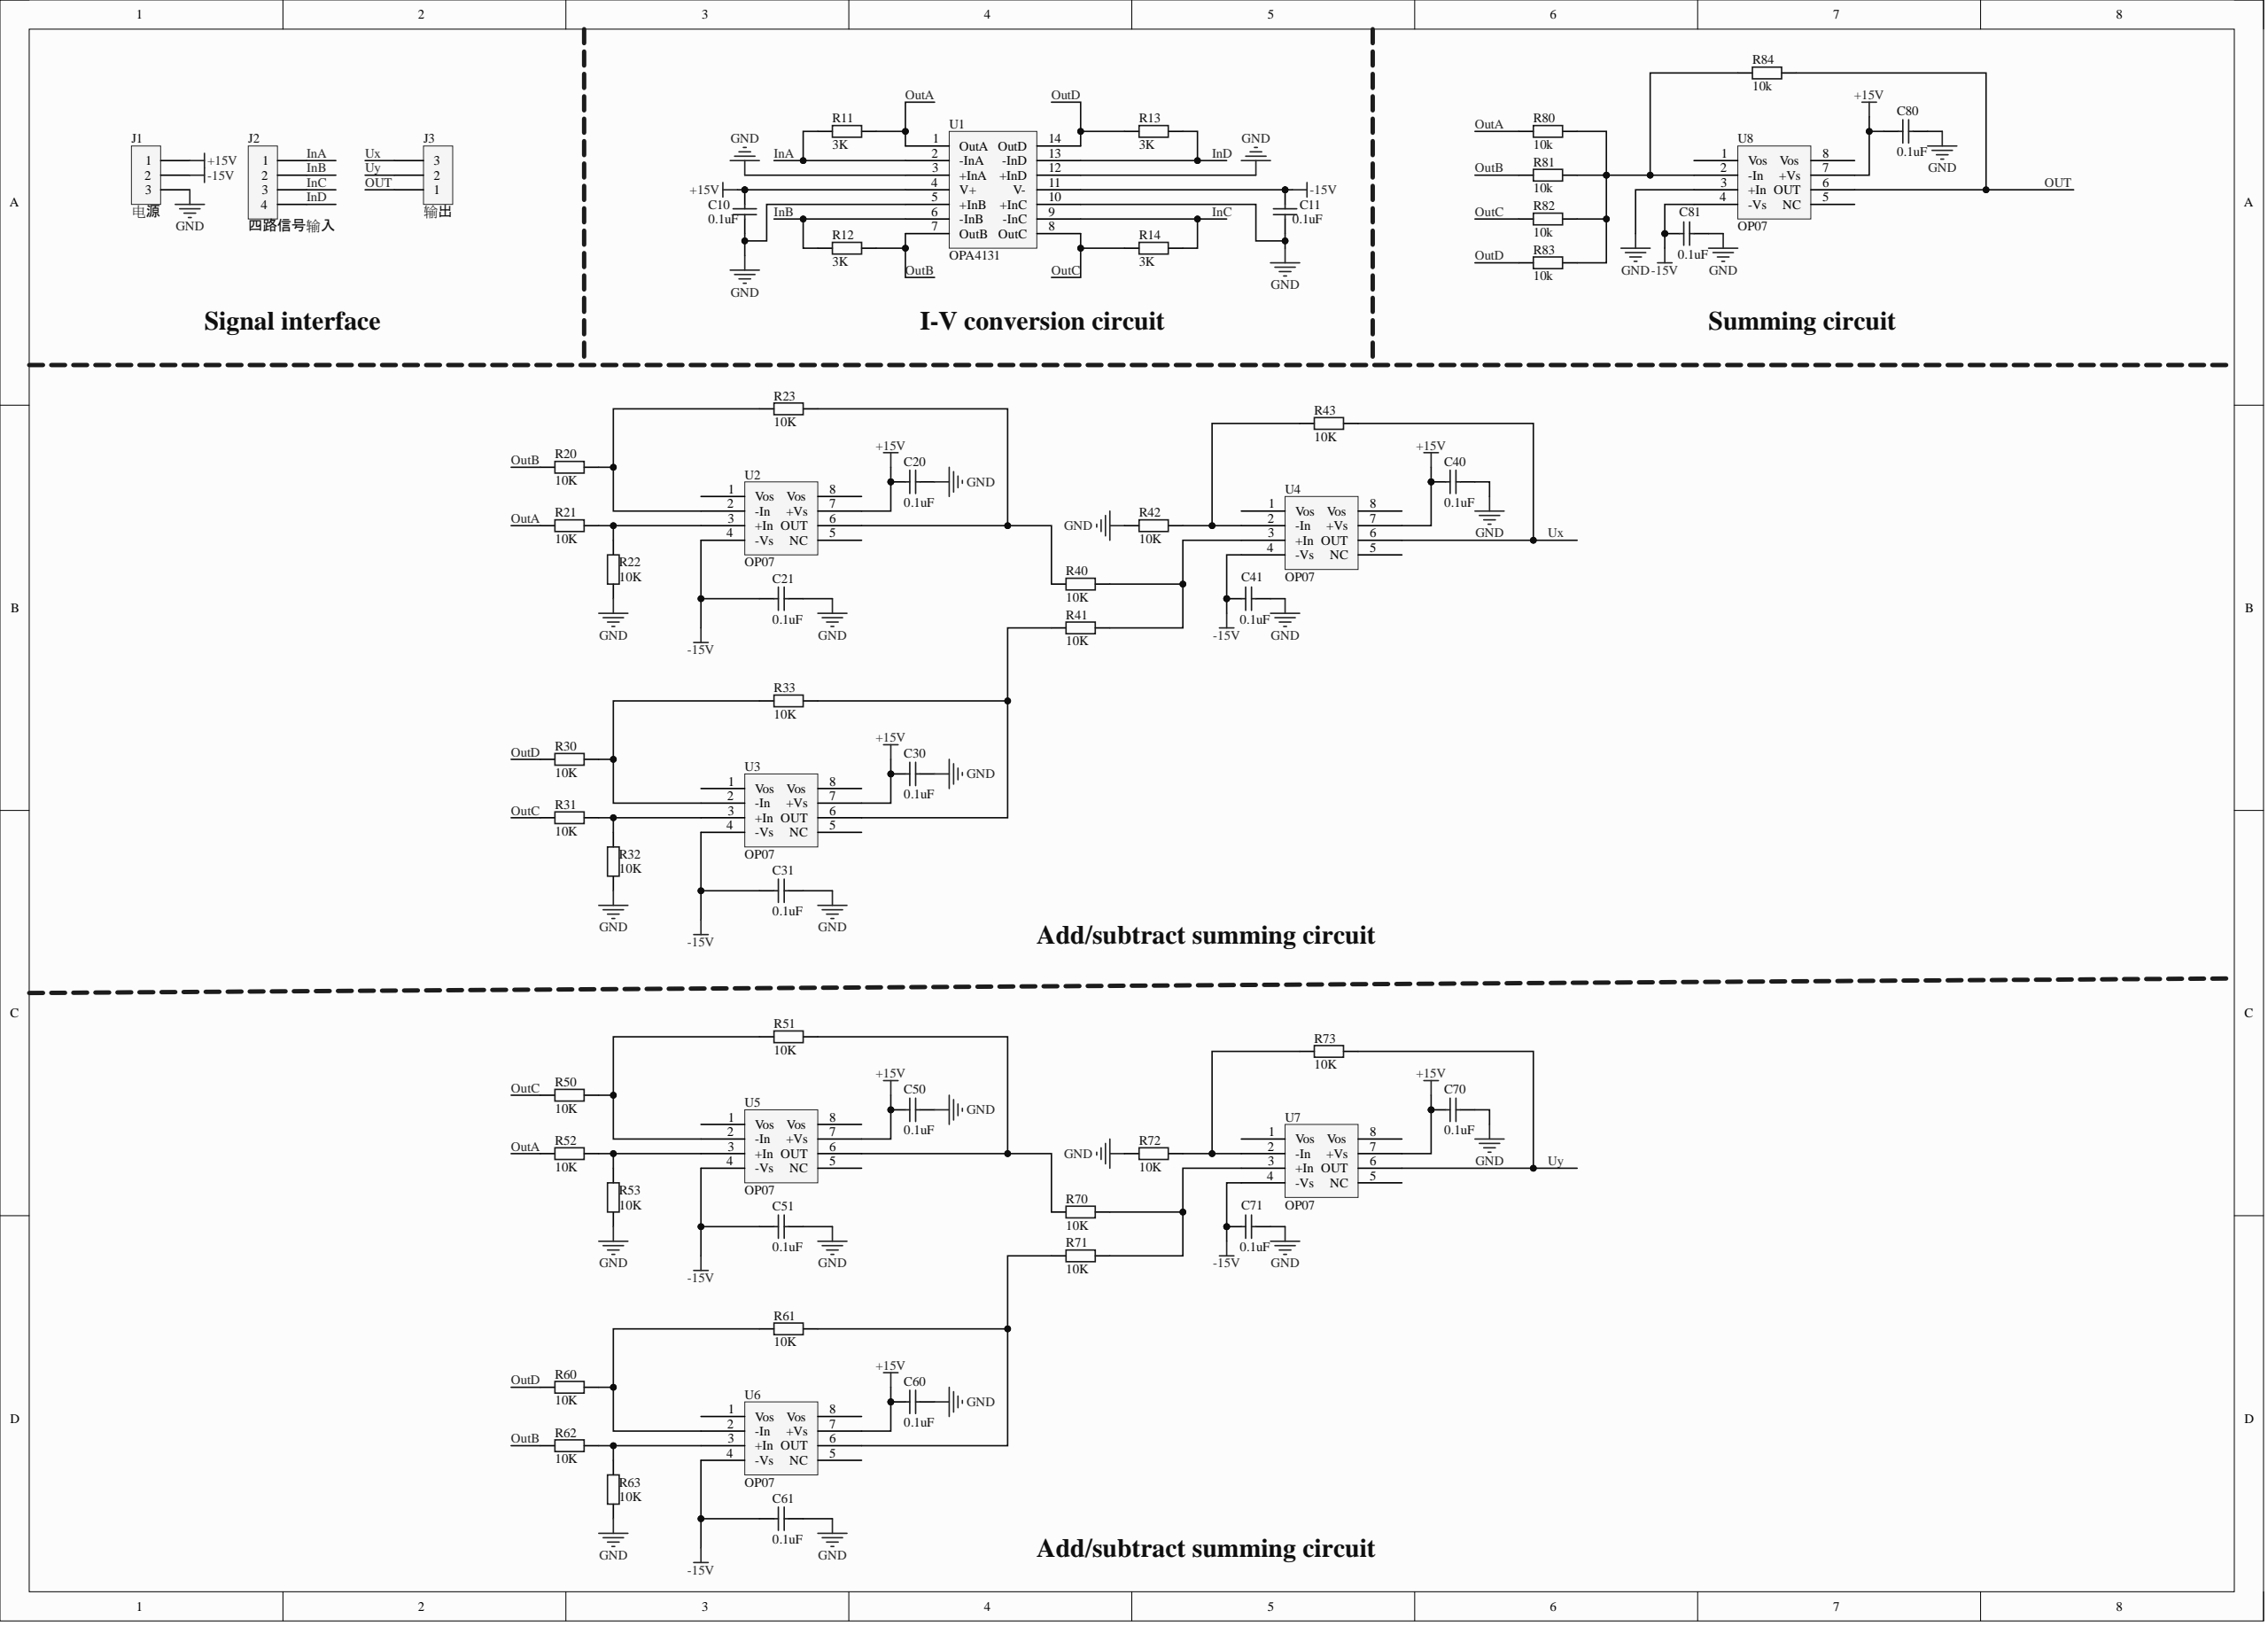Circuit board | Altium Designer | 60 parts | 31 nets
Bill of materials:
Comment,Description,Designator,Footprint,LibRef,Quantity
"0.1uF","Capacitor","C10, C11, C20, C21, C30, C31, C40, C41, C50, C51, C60, C61, C70, C71, C80, C81","C0805","Cap","16"
"电源","","J1","HDR1X3","电源","1"
"四路信号输入","","J2","HDR1X4","CON4","1"
"输出","","J3","HDR1X3","电源","1"
"3K","Resistor","R11, R12, R13, R14","R0805","Res2","4"
"10K","Resistor","R20, R21, R22, R23, R30, R31, R32, R33, R40, R41, R42, R43, R50, R51, R52, R53, R60, R61, R62, R63, R70, R71, R72, R73, R80, R81, R82, R83, R84","R0805","Res2","29"
"OPA4131","","U1","SOIC-14_L8.7-W3.9-P1.27-LS6.0-BL","OPA4131","1"
"OP07","","U2, U3, U4, U5, U6, U7, U8","SOP-8_L4.9-W3.9-P1.27-LS6.0-BL","OP07","7"
Netlist (Protel format):
[
C10
C0805
0.1uF



]
[
C11
C0805
0.1uF



]
[
C20
C0805
0.1uF



]
[
C21
C0805
0.1uF



]
[
C30
C0805
0.1uF



]
[
C31
C0805
0.1uF



]
[
C40
C0805
0.1uF



]
[
C41
C0805
0.1uF



]
[
C50
C0805
0.1uF



]
[
C51
C0805
0.1uF



]
[
C60
C0805
0.1uF



]
[
C61
C0805
0.1uF



]
[
C70
C0805
0.1uF



]
[
C71
C0805
0.1uF



]
[
C80
C0805
0.1uF



]
[
C81
C0805
0.1uF



]
[
J1
HDR1X3
电源



]
[
J2
HDR1X4
四路信号输入



]
[
J3
HDR1X3
输出



]
[
R11
R0805
3K



]
[
R12
R0805
3K



]
[
R13
R0805
3K



]
[
R14
R0805
3K



]
[
R20
R0805
10K



]
[
R21
R0805
10K



]
[
R22
R0805
10K



]
[
R23
R0805
10K



]
[
R30
R0805
10K



]
[
R31
R0805
10K



]
[
R32
R0805
10K



]
[
R33
R0805
10K



]
[
R40
R0805
10K



]
[
R41
R0805
10K



]
[
R42
R0805
10K



]
[
R43
R0805
10K



]
[
R50
R0805
10K



]
[
R51
R0805
10K



]
[
R52
R0805
10K



]
[
R53
R0805
10K



]
[
R60
R0805
10K



]
[
R61
R0805
10K



]
[
R62
R0805
10K



]
[
R63
R0805
10K



]
[
R70
R0805
10K



]
[
R71
R0805
10K



]
[
R72
R0805
10K



]
[
R73
R0805
10K



]
[
R80
R0805
10k



]
[
R81
R0805
10k



]
[
R82
R0805
10k



]
[
R83
R0805
10k



]
[
R84
R0805
10k



]
[
U1
SOIC-14_L8.7-W3.9-P1.27-LS6.0-BL
OPA4131



]
[
U2
SOP-8_L4.9-W3.9-P1.27-LS6.0-BL
OP07



]
[
U3
SOP-8_L4.9-W3.9-P1.27-LS6.0-BL
OP07



]
[
U4
SOP-8_L4.9-W3.9-P1.27-LS6.0-BL
OP07



]
[
U5
SOP-8_L4.9-W3.9-P1.27-LS6.0-BL
OP07



]
[
U6
SOP-8_L4.9-W3.9-P1.27-LS6.0-BL
OP07



]
[
U7
SOP-8_L4.9-W3.9-P1.27-LS6.0-BL
OP07



]
[
U8
SOP-8_L4.9-W3.9-P1.27-LS6.0-BL
OP07



]
(
Uy
J3-2
R73-1
U7-6
)
(
Ux
J3-3
R43-1
U4-6
)
(
OutD
R13-1
R30-1
R60-1
R83-1
U1-14
)
(
OutC
R14-1
R31-1
R50-1
R82-1
U1-8
)
(
OutB
R12-2
R20-1
R62-1
R81-1
U1-7
)
(
OutA
R11-2
R21-1
R52-1
R80-1
U1-1
)
(
OUT
J3-1
R84-2
U8-6
)
(
NetR80_2
R80-2
R81-2
R82-2
R83-2
R84-1
U8-2
)
(
NetR72_2
R72-2
R73-2
U7-2
)
(
NetR70_2
R70-2
R71-2
U7-3
)
(
NetR62_2
R62-2
R63-2
U6-3
)
(
NetR61_2
R61-2
R71-1
U6-6
)
(
NetR60_2
R60-2
R61-1
U6-2
)
(
NetR52_2
R52-2
R53-2
U5-3
)
(
NetR51_2
R51-2
R70-1
U5-6
)
(
NetR50_2
R50-2
R51-1
U5-2
)
(
NetR42_2
R42-2
R43-2
U4-2
)
(
NetR40_2
R40-2
R41-2
U4-3
)
(
NetR33_2
R33-2
R41-1
U3-6
)
(
NetR31_2
R31-2
R32-2
U3-3
)
(
NetR30_2
R30-2
R33-1
U3-2
)
(
NetR23_2
R23-2
R40-1
U2-6
)
(
NetR21_2
R21-2
R22-2
U2-3
)
(
NetR20_2
R20-2
R23-1
U2-2
)
(
InD
J2-4
R13-2
U1-13
)
(
InC
J2-3
R14-2
U1-9
)
(
InB
J2-2
R12-1
U1-6
)
(
InA
J2-1
R11-1
U1-2
)
(
GND
C10-1
C11-1
C20-2
C21-2
C30-2
C31-2
C40-2
C41-2
C50-2
C51-2
C60-2
C61-2
C70-2
C71-2
C80-2
C81-2
J1-3
R22-1
R32-1
R42-1
R53-1
R63-1
R72-1
U1-3
U1-5
U1-10
U1-12
U8-3
)
(
-15V
C11-2
C21-1
C31-1
C41-1
C51-1
C61-1
C71-1
C81-1
J1-2
U1-11
U2-4
U3-4
U4-4
U5-4
U6-4
U7-4
U8-4
)
(
+15V
C10-2
C20-1
C30-1
C40-1
C50-1
C60-1
C70-1
C80-1
J1-1
U1-4
U2-7
U3-7
U4-7
U5-7
U6-7
U7-7
U8-7
)